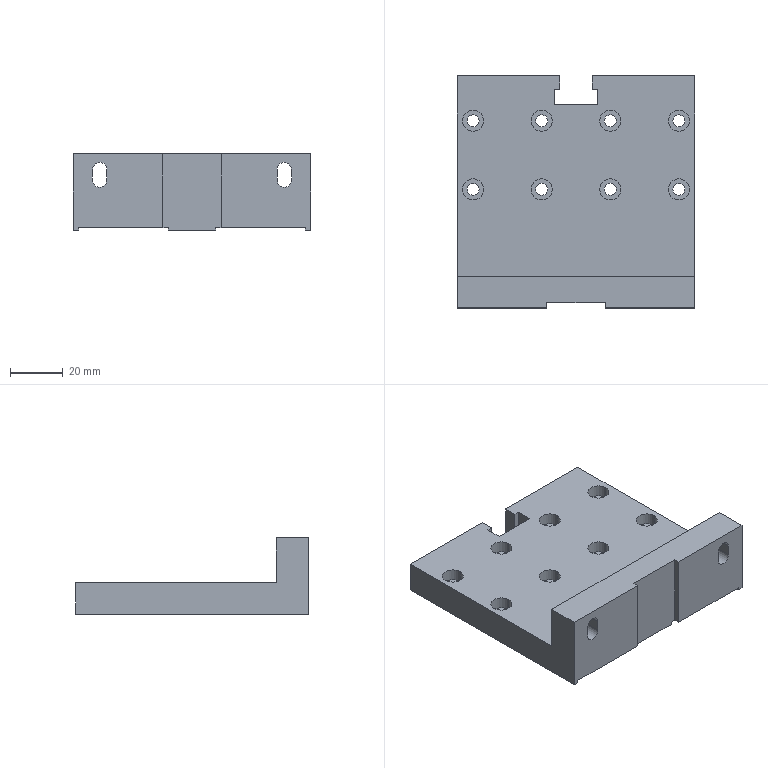Part | STEP file | 2049 Bag feed connecting plate 2 | 1 solid | 78 faces | box 90 x 88 x 29 mm | volume 100448 mm3 | plane 40 | cylinder 38 | commonest cylinder face diameters 4.5 x16 8 x16 5.5 x6